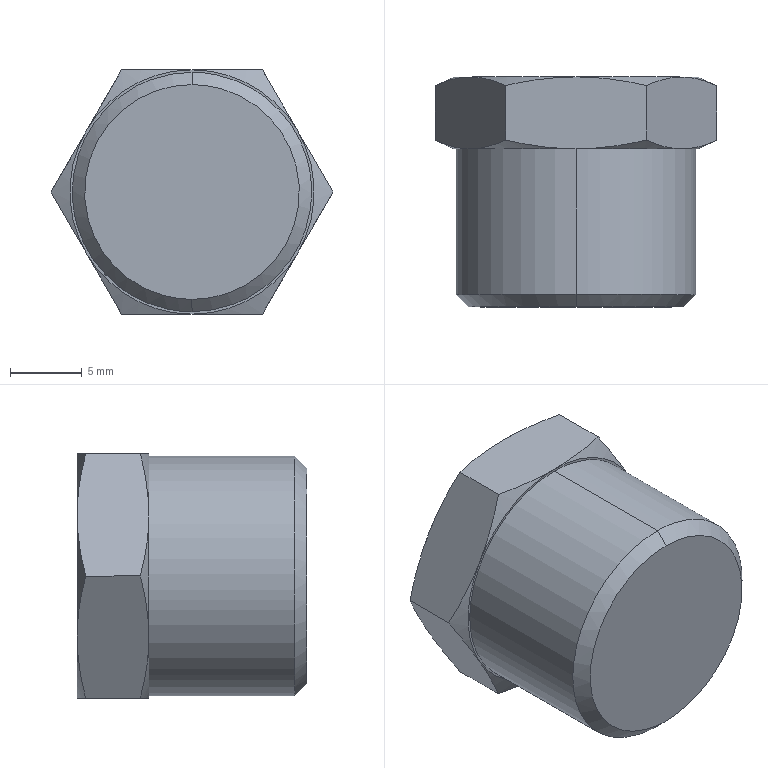Part | SolidWorks | features BaseBody 1 | 1 solid | 25 faces | box 19.63 x 16 x 17 mm | volume 3623 mm3 | cone 14 | plane 9 | cylinder 2 | commonest cylinder face diameters 16.662 x2
STEP:
#1=CARTESIAN_POINT('',(0.,0.,-7.475));
#2=VERTEX_POINT('',#1);
#3=CARTESIAN_POINT('',(0.,0.,7.475));
#4=VERTEX_POINT('',#3);
#5=CARTESIAN_POINT('',(0.,0.,-7.475));
#6=CARTESIAN_POINT('',(0.4908,0.,-7.475));
#7=CARTESIAN_POINT('',(0.9769,0.,-7.427));
#8=CARTESIAN_POINT('',(1.94,0.,-7.236));
#9=CARTESIAN_POINT('',(2.407,0.,-7.094));
#10=CARTESIAN_POINT('',(3.314,0.,-6.718));
#11=CARTESIAN_POINT('',(3.745,0.,-6.488));
#12=CARTESIAN_POINT('',(4.561,0.,-5.943));
#13=CARTESIAN_POINT('',(4.939,0.,-5.633));
#14=CARTESIAN_POINT('',(5.633,0.,-4.939));
#15=CARTESIAN_POINT('',(5.943,0.,-4.561));
#16=CARTESIAN_POINT('',(6.488,0.,-3.745));
#17=CARTESIAN_POINT('',(6.718,0.,-3.314));
#18=CARTESIAN_POINT('',(7.094,0.,-2.407));
#19=CARTESIAN_POINT('',(7.236,0.,-1.94));
#20=CARTESIAN_POINT('',(7.427,0.,-0.9769));
#21=CARTESIAN_POINT('',(7.475,0.,-0.4908));
#22=CARTESIAN_POINT('',(7.475,0.,0.4908));
#23=CARTESIAN_POINT('',(7.427,0.,0.9769));
#24=CARTESIAN_POINT('',(7.236,0.,1.94));
#25=CARTESIAN_POINT('',(7.094,0.,2.407));
#26=CARTESIAN_POINT('',(6.718,0.,3.314));
#27=CARTESIAN_POINT('',(6.488,0.,3.745));
#28=CARTESIAN_POINT('',(5.943,0.,4.561));
#29=CARTESIAN_POINT('',(5.633,0.,4.939));
#30=CARTESIAN_POINT('',(4.939,0.,5.633));
#31=CARTESIAN_POINT('',(4.561,0.,5.943));
#32=CARTESIAN_POINT('',(3.745,0.,6.488));
#33=CARTESIAN_POINT('',(3.314,0.,6.718));
#34=CARTESIAN_POINT('',(2.407,0.,7.094));
#35=CARTESIAN_POINT('',(1.94,0.,7.236));
#36=CARTESIAN_POINT('',(0.9769,0.,7.427));
#37=CARTESIAN_POINT('',(0.4908,0.,7.475));
#38=CARTESIAN_POINT('',(0.,0.,7.475));
#39=B_SPLINE_CURVE_WITH_KNOTS('',3,(#5,#6,#7,#8,#9,#10,#11,#12,#13,#14,#15,#16,#17,#18,#19,#20,#21,#22,#23,#24,#25,#26,#27,#28,#29,#30,#31,#32,#33,#34,#35,#36,#37,#38),.UNSPECIFIED.,.F.,.F.,(4,2,2,2,2,2,2,2,2,2,2,2,2,2,2,2,4),(0.,0.1963,0.3927,0.589,0.7854,0.9817,1.178,1.374,1.571,1.767,1.963,2.16,2.356,2.553,2.749,2.945,3.142),.UNSPECIFIED.);
#40=EDGE_CURVE('',#2,#4,#39,.T.);
#41=ORIENTED_EDGE('',*,*,#40,.F.);
#42=CARTESIAN_POINT('',(0.,0.856,-8.331));
#43=VERTEX_POINT('',#42);
#44=CARTESIAN_POINT('',(0.,0.856,-8.331));
#45=DIRECTION('',(0.,0.7071,-0.7071));
#46=VECTOR('',#45,1000.);
#47=LINE('',#44,#46);
#48=EDGE_CURVE('',#2,#43,#47,.T.);
#49=ORIENTED_EDGE('',*,*,#48,.T.);
#50=CARTESIAN_POINT('',(0.,0.856,8.331));
#51=VERTEX_POINT('',#50);
#52=CARTESIAN_POINT('',(0.,0.856,-8.331));
#53=CARTESIAN_POINT('',(1.091,0.856,-8.331));
#54=CARTESIAN_POINT('',(2.181,0.856,-8.114));
#55=CARTESIAN_POINT('',(4.196,0.856,-7.28));
#56=CARTESIAN_POINT('',(5.12,0.856,-6.662));
#57=CARTESIAN_POINT('',(6.662,0.856,-5.12));
#58=CARTESIAN_POINT('',(7.28,0.856,-4.196));
#59=CARTESIAN_POINT('',(8.114,0.856,-2.181));
#60=CARTESIAN_POINT('',(8.331,0.856,-1.091));
#61=CARTESIAN_POINT('',(8.331,0.856,1.091));
#62=CARTESIAN_POINT('',(8.114,0.856,2.181));
#63=CARTESIAN_POINT('',(7.28,0.856,4.196));
#64=CARTESIAN_POINT('',(6.662,0.856,5.12));
#65=CARTESIAN_POINT('',(5.12,0.856,6.662));
#66=CARTESIAN_POINT('',(4.196,0.856,7.28));
#67=CARTESIAN_POINT('',(2.181,0.856,8.114));
#68=CARTESIAN_POINT('',(1.091,0.856,8.331));
#69=CARTESIAN_POINT('',(0.,0.856,8.331));
#70=B_SPLINE_CURVE_WITH_KNOTS('',3,(#52,#53,#54,#55,#56,#57,#58,#59,#60,#61,#62,#63,#64,#65,#66,#67,#68,#69),.UNSPECIFIED.,.F.,.F.,(4,2,2,2,2,2,2,2,4),(0.,0.3927,0.7854,1.178,1.571,1.963,2.356,2.749,3.142),.UNSPECIFIED.);
#71=EDGE_CURVE('',#43,#51,#70,.T.);
#72=ORIENTED_EDGE('',*,*,#71,.T.);
#73=CARTESIAN_POINT('',(0.,0.856,8.331));
#74=DIRECTION('',(0.,0.7071,0.7071));
#75=VECTOR('',#74,1000.);
#76=LINE('',#73,#75);
#77=EDGE_CURVE('',#4,#51,#76,.T.);
#78=ORIENTED_EDGE('',*,*,#77,.F.);
#79=EDGE_LOOP('',(#41,#49,#72,#78));
#80=FACE_OUTER_BOUND('',#79,.T.);
#81=CARTESIAN_POINT('',(0.,0.856,0.));
#82=DIRECTION('',(0.,1.,0.));
#83=DIRECTION('',(0.,0.,1.));
#84=AXIS2_PLACEMENT_3D('',#81,#82,#83);
#85=CONICAL_SURFACE('',#84,8.331,0.7854);
#86=ADVANCED_FACE('',(#80),#85,.T.);
#87=CARTESIAN_POINT('',(0.,11.,-8.331));
#88=VERTEX_POINT('',#87);
#89=CARTESIAN_POINT('',(0.,11.,8.331));
#90=VERTEX_POINT('',#89);
#91=CARTESIAN_POINT('',(0.,11.,-8.331));
#92=CARTESIAN_POINT('',(1.091,11.,-8.331));
#93=CARTESIAN_POINT('',(2.181,11.,-8.114));
#94=CARTESIAN_POINT('',(4.196,11.,-7.28));
#95=CARTESIAN_POINT('',(5.12,11.,-6.662));
#96=CARTESIAN_POINT('',(6.662,11.,-5.12));
#97=CARTESIAN_POINT('',(7.28,11.,-4.196));
#98=CARTESIAN_POINT('',(8.114,11.,-2.181));
#99=CARTESIAN_POINT('',(8.331,11.,-1.091));
#100=CARTESIAN_POINT('',(8.331,11.,1.091));
#101=CARTESIAN_POINT('',(8.114,11.,2.181));
#102=CARTESIAN_POINT('',(7.28,11.,4.196));
#103=CARTESIAN_POINT('',(6.662,11.,5.12));
#104=CARTESIAN_POINT('',(5.12,11.,6.662));
#105=CARTESIAN_POINT('',(4.196,11.,7.28));
#106=CARTESIAN_POINT('',(2.181,11.,8.114));
#107=CARTESIAN_POINT('',(1.091,11.,8.331));
#108=CARTESIAN_POINT('',(0.,11.,8.331));
#109=B_SPLINE_CURVE_WITH_KNOTS('',3,(#91,#92,#93,#94,#95,#96,#97,#98,#99,#100,#101,#102,#103,#104,#105,#106,#107,#108),.UNSPECIFIED.,.F.,.F.,(4,2,2,2,2,2,2,2,4),(0.,0.3927,0.7854,1.178,1.571,1.963,2.356,2.749,3.142),.UNSPECIFIED.);
#110=EDGE_CURVE('',#88,#90,#109,.T.);
#111=ORIENTED_EDGE('',*,*,#110,.T.);
#112=CARTESIAN_POINT('',(0.,0.,8.331));
#113=DIRECTION('',(0.,-1.,0.));
#114=VECTOR('',#113,1000.);
#115=LINE('',#112,#114);
#116=EDGE_CURVE('',#90,#51,#115,.T.);
#117=ORIENTED_EDGE('',*,*,#116,.T.);
#118=ORIENTED_EDGE('',*,*,#71,.F.);
#119=CARTESIAN_POINT('',(0.,0.,-8.331));
#120=DIRECTION('',(0.,-1.,0.));
#121=VECTOR('',#120,1000.);
#122=LINE('',#119,#121);
#123=EDGE_CURVE('',#88,#43,#122,.T.);
#124=ORIENTED_EDGE('',*,*,#123,.F.);
#125=EDGE_LOOP('',(#111,#117,#118,#124));
#126=FACE_OUTER_BOUND('',#125,.T.);
#127=CARTESIAN_POINT('',(0.,0.,0.));
#128=DIRECTION('',(0.,-1.,0.));
#129=DIRECTION('',(0.,0.,-1.));
#130=AXIS2_PLACEMENT_3D('',#127,#128,#129);
#131=CYLINDRICAL_SURFACE('',#130,8.331);
#132=ADVANCED_FACE('',(#126),#131,.T.);
#133=CARTESIAN_POINT('',(-7.361,11.,4.25));
#134=VERTEX_POINT('',#133);
#135=CARTESIAN_POINT('',(-9.815,11.599,0.));
#136=VERTEX_POINT('',#135);
#137=CARTESIAN_POINT('',(-7.361,11.,4.25));
#138=CARTESIAN_POINT('',(-7.562,11.,3.903));
#139=CARTESIAN_POINT('',(-7.761,11.012,3.556));
#140=CARTESIAN_POINT('',(-8.067,11.052,3.027));
#141=CARTESIAN_POINT('',(-8.169,11.068,2.849));
#142=CARTESIAN_POINT('',(-8.326,11.098,2.578));
#143=CARTESIAN_POINT('',(-8.405,11.115,2.442));
#144=CARTESIAN_POINT('',(-8.498,11.136,2.281));
#145=CARTESIAN_POINT('',(-8.538,11.146,2.212));
#146=CARTESIAN_POINT('',(-8.565,11.152,2.165));
#147=CARTESIAN_POINT('',(-8.579,11.156,2.141));
#148=CARTESIAN_POINT('',(-8.968,11.254,1.466));
#149=CARTESIAN_POINT('',(-9.366,11.395,0.7774));
#150=CARTESIAN_POINT('',(-9.815,11.599,0.));
#151=B_SPLINE_CURVE_WITH_KNOTS('',3,(#137,#138,#139,#140,#141,#142,#143,#144,#145,#146,#147,#148,#149,#150),.UNSPECIFIED.,.F.,.F.,(4,2,2,1,1,2,2,4),(4.934,6.158,6.77,7.075,7.228,7.305,7.381,9.828),.UNSPECIFIED.);
#152=EDGE_CURVE('',#134,#136,#151,.T.);
#153=ORIENTED_EDGE('',*,*,#152,.T.);
#154=CARTESIAN_POINT('',(-7.361,11.,-4.25));
#155=VERTEX_POINT('',#154);
#156=CARTESIAN_POINT('',(-9.815,11.599,0.));
#157=CARTESIAN_POINT('',(-9.59,11.497,-0.3897));
#158=CARTESIAN_POINT('',(-9.378,11.411,-0.7558));
#159=CARTESIAN_POINT('',(-9.074,11.302,-1.282));
#160=CARTESIAN_POINT('',(-8.976,11.269,-1.453));
#161=CARTESIAN_POINT('',(-8.83,11.225,-1.705));
#162=CARTESIAN_POINT('',(-8.758,11.203,-1.83));
#163=CARTESIAN_POINT('',(-8.675,11.181,-1.974));
#164=CARTESIAN_POINT('',(-8.634,11.17,-2.046));
#165=CARTESIAN_POINT('',(-8.616,11.165,-2.076));
#166=CARTESIAN_POINT('',(-8.604,11.162,-2.097));
#167=CARTESIAN_POINT('',(-8.599,11.161,-2.105));
#168=CARTESIAN_POINT('',(-8.161,11.05,-2.864));
#169=CARTESIAN_POINT('',(-7.762,11.,-3.556));
#170=CARTESIAN_POINT('',(-7.361,11.,-4.25));
#171=B_SPLINE_CURVE_WITH_KNOTS('',3,(#156,#157,#158,#159,#160,#161,#162,#163,#164,#165,#166,#167,#168,#169,#170),.UNSPECIFIED.,.F.,.F.,(4,2,2,1,1,1,2,2,4),(0.0002337,1.234,1.85,2.159,2.313,2.39,2.429,2.467,4.934),.UNSPECIFIED.);
#172=EDGE_CURVE('',#136,#155,#171,.T.);
#173=ORIENTED_EDGE('',*,*,#172,.T.);
#174=CARTESIAN_POINT('',(0.,11.,0.));
#175=DIRECTION('',(0.,-1.,0.));
#176=DIRECTION('',(-0.866,0.,0.5));
#177=AXIS2_PLACEMENT_3D('',#174,#175,#176);
#178=CIRCLE('',#177,8.5);
#179=EDGE_CURVE('',#134,#155,#178,.T.);
#180=ORIENTED_EDGE('',*,*,#179,.F.);
#181=EDGE_LOOP('',(#153,#173,#180));
#182=FACE_OUTER_BOUND('',#181,.T.);
#183=CARTESIAN_POINT('',(0.,11.599,0.));
#184=DIRECTION('',(0.,1.,0.));
#185=DIRECTION('',(0.,0.,1.));
#186=AXIS2_PLACEMENT_3D('',#183,#184,#185);
#187=CONICAL_SURFACE('',#186,9.815,1.143);
#188=ADVANCED_FACE('',(#182),#187,.T.);
#189=CARTESIAN_POINT('',(0.,11.,-8.5));
#190=VERTEX_POINT('',#189);
#191=CARTESIAN_POINT('',(0.,11.,0.));
#192=DIRECTION('',(0.,-1.,0.));
#193=DIRECTION('',(-0.866,0.,-0.5));
#194=AXIS2_PLACEMENT_3D('',#191,#192,#193);
#195=CIRCLE('',#194,8.5);
#196=EDGE_CURVE('',#155,#190,#195,.T.);
#197=ORIENTED_EDGE('',*,*,#196,.F.);
#198=CARTESIAN_POINT('',(-4.907,11.599,-8.5));
#199=VERTEX_POINT('',#198);
#200=CARTESIAN_POINT('',(-7.361,11.,-4.25));
#201=CARTESIAN_POINT('',(-7.161,11.,-4.597));
#202=CARTESIAN_POINT('',(-6.96,11.012,-4.943));
#203=CARTESIAN_POINT('',(-6.655,11.052,-5.473));
#204=CARTESIAN_POINT('',(-6.552,11.068,-5.651));
#205=CARTESIAN_POINT('',(-6.396,11.098,-5.921));
#206=CARTESIAN_POINT('',(-6.317,11.115,-6.058));
#207=CARTESIAN_POINT('',(-6.224,11.136,-6.219));
#208=CARTESIAN_POINT('',(-6.184,11.146,-6.288));
#209=CARTESIAN_POINT('',(-6.158,11.152,-6.335));
#210=CARTESIAN_POINT('',(-6.143,11.156,-6.359));
#211=CARTESIAN_POINT('',(-5.754,11.254,-7.033));
#212=CARTESIAN_POINT('',(-5.356,11.395,-7.723));
#213=CARTESIAN_POINT('',(-4.907,11.599,-8.5));
#214=B_SPLINE_CURVE_WITH_KNOTS('',3,(#200,#201,#202,#203,#204,#205,#206,#207,#208,#209,#210,#211,#212,#213),.UNSPECIFIED.,.F.,.F.,(4,2,2,1,1,2,2,4),(4.934,6.158,6.77,7.075,7.228,7.305,7.381,9.828),.UNSPECIFIED.);
#215=EDGE_CURVE('',#155,#199,#214,.T.);
#216=ORIENTED_EDGE('',*,*,#215,.T.);
#217=CARTESIAN_POINT('',(-4.907,11.599,-8.5));
#218=CARTESIAN_POINT('',(-4.475,11.501,-8.5));
#219=CARTESIAN_POINT('',(-4.068,11.418,-8.5));
#220=CARTESIAN_POINT('',(-3.628,11.338,-8.5));
#221=CARTESIAN_POINT('',(-3.579,11.329,-8.5));
#222=CARTESIAN_POINT('',(-3.482,11.312,-8.5));
#223=CARTESIAN_POINT('',(-3.425,11.303,-8.5));
#224=CARTESIAN_POINT('',(-3.264,11.276,-8.5));
#225=CARTESIAN_POINT('',(-3.158,11.258,-8.5));
#226=CARTESIAN_POINT('',(-2.843,11.21,-8.5));
#227=CARTESIAN_POINT('',(-2.637,11.181,-8.5));
#228=CARTESIAN_POINT('',(-2.232,11.13,-8.5));
#229=CARTESIAN_POINT('',(-2.034,11.108,-8.5));
#230=CARTESIAN_POINT('',(-1.788,11.085,-8.5));
#231=CARTESIAN_POINT('',(-1.738,11.08,-8.5));
#232=CARTESIAN_POINT('',(-1.634,11.071,-8.5));
#233=CARTESIAN_POINT('',(-1.477,11.058,-8.5));
#234=CARTESIAN_POINT('',(-1.322,11.046,-8.5));
#235=CARTESIAN_POINT('',(-0.8077,11.013,-8.5));
#236=CARTESIAN_POINT('',(-0.4041,11.,-8.5));
#237=CARTESIAN_POINT('',(0.,11.,-8.5));
#238=B_SPLINE_CURVE_WITH_KNOTS('',3,(#217,#218,#219,#220,#221,#222,#223,#224,#225,#226,#227,#228,#229,#230,#231,#232,#233,#234,#235,#236,#237),.UNSPECIFIED.,.F.,.F.,(4,2,2,2,2,2,2,2,1,2,4),(10.366,11.605,11.76,11.915,12.225,12.845,13.465,13.62,13.775,14.085,15.324),.UNSPECIFIED.);
#239=EDGE_CURVE('',#199,#190,#238,.T.);
#240=ORIENTED_EDGE('',*,*,#239,.T.);
#241=EDGE_LOOP('',(#197,#216,#240));
#242=FACE_OUTER_BOUND('',#241,.T.);
#243=CARTESIAN_POINT('',(0.,11.599,0.));
#244=DIRECTION('',(0.,1.,0.));
#245=DIRECTION('',(0.,0.,1.));
#246=AXIS2_PLACEMENT_3D('',#243,#244,#245);
#247=CONICAL_SURFACE('',#246,9.815,1.143);
#248=ADVANCED_FACE('',(#242),#247,.T.);
#249=CARTESIAN_POINT('',(7.361,11.,-4.25));
#250=VERTEX_POINT('',#249);
#251=CARTESIAN_POINT('',(0.,11.,0.));
#252=DIRECTION('',(0.,-1.,0.));
#253=DIRECTION('',(0.,0.,-1.));
#254=AXIS2_PLACEMENT_3D('',#251,#252,#253);
#255=CIRCLE('',#254,8.5);
#256=EDGE_CURVE('',#190,#250,#255,.T.);
#257=ORIENTED_EDGE('',*,*,#256,.F.);
#258=CARTESIAN_POINT('',(4.907,11.599,-8.5));
#259=VERTEX_POINT('',#258);
#260=CARTESIAN_POINT('',(0.,11.,-8.5));
#261=CARTESIAN_POINT('',(0.4009,11.,-8.5));
#262=CARTESIAN_POINT('',(0.8009,11.012,-8.499));
#263=CARTESIAN_POINT('',(1.412,11.052,-8.499));
#264=CARTESIAN_POINT('',(1.617,11.068,-8.499));
#265=CARTESIAN_POINT('',(1.93,11.098,-8.5));
#266=CARTESIAN_POINT('',(2.087,11.115,-8.5));
#267=CARTESIAN_POINT('',(2.273,11.136,-8.5));
#268=CARTESIAN_POINT('',(2.367,11.147,-8.5));
#269=CARTESIAN_POINT('',(2.407,11.152,-8.5));
#270=CARTESIAN_POINT('',(2.434,11.156,-8.5));
#271=CARTESIAN_POINT('',(2.448,11.157,-8.5));
#272=CARTESIAN_POINT('',(2.657,11.184,-8.5));
#273=CARTESIAN_POINT('',(2.857,11.212,-8.5));
#274=CARTESIAN_POINT('',(3.163,11.259,-8.5));
#275=CARTESIAN_POINT('',(3.317,11.284,-8.5));
#276=CARTESIAN_POINT('',(3.5,11.315,-8.5));
#277=CARTESIAN_POINT('',(3.579,11.329,-8.5));
#278=CARTESIAN_POINT('',(3.632,11.339,-8.5));
#279=CARTESIAN_POINT('',(3.66,11.344,-8.5));
#280=CARTESIAN_POINT('',(3.785,11.366,-8.5));
#281=CARTESIAN_POINT('',(3.936,11.395,-8.5));
#282=CARTESIAN_POINT('',(4.089,11.425,-8.5));
#283=CARTESIAN_POINT('',(4.193,11.446,-8.5));
#284=CARTESIAN_POINT('',(4.246,11.456,-8.5));
#285=CARTESIAN_POINT('',(4.397,11.487,-8.5));
#286=CARTESIAN_POINT('',(4.501,11.509,-8.5));
#287=CARTESIAN_POINT('',(4.703,11.553,-8.5));
#288=CARTESIAN_POINT('',(4.805,11.576,-8.5));
#289=CARTESIAN_POINT('',(4.907,11.599,-8.5));
#290=B_SPLINE_CURVE_WITH_KNOTS('',3,(#260,#261,#262,#263,#264,#265,#266,#267,#268,#269,#270,#271,#272,#273,#274,#275,#276,#277,#278,#279,#280,#281,#282,#283,#284,#285,#286,#287,#288,#289),.UNSPECIFIED.,.F.,.F.,(4,2,2,1,1,1,2,2,2,1,1,2,2,1,2,2,2,4),(15.324,16.571,17.194,17.506,17.662,17.74,17.779,17.818,18.441,18.753,18.909,18.987,19.065,19.376,19.532,19.688,20.,20.311),.UNSPECIFIED.);
#291=EDGE_CURVE('',#190,#259,#290,.T.);
#292=ORIENTED_EDGE('',*,*,#291,.T.);
#293=CARTESIAN_POINT('',(4.907,11.599,-8.5));
#294=CARTESIAN_POINT('',(5.132,11.497,-8.11));
#295=CARTESIAN_POINT('',(5.343,11.411,-7.744));
#296=CARTESIAN_POINT('',(5.647,11.302,-7.218));
#297=CARTESIAN_POINT('',(5.746,11.269,-7.047));
#298=CARTESIAN_POINT('',(5.892,11.225,-6.794));
#299=CARTESIAN_POINT('',(5.964,11.203,-6.67));
#300=CARTESIAN_POINT('',(6.047,11.181,-6.526));
#301=CARTESIAN_POINT('',(6.089,11.17,-6.454));
#302=CARTESIAN_POINT('',(6.106,11.165,-6.424));
#303=CARTESIAN_POINT('',(6.118,11.162,-6.403));
#304=CARTESIAN_POINT('',(6.123,11.161,-6.395));
#305=CARTESIAN_POINT('',(6.561,11.05,-5.636));
#306=CARTESIAN_POINT('',(6.96,11.,-4.944));
#307=CARTESIAN_POINT('',(7.361,11.,-4.25));
#308=B_SPLINE_CURVE_WITH_KNOTS('',3,(#293,#294,#295,#296,#297,#298,#299,#300,#301,#302,#303,#304,#305,#306,#307),.UNSPECIFIED.,.F.,.F.,(4,2,2,1,1,1,2,2,4),(0.0002337,1.234,1.85,2.159,2.313,2.39,2.429,2.467,4.934),.UNSPECIFIED.);
#309=EDGE_CURVE('',#259,#250,#308,.T.);
#310=ORIENTED_EDGE('',*,*,#309,.T.);
#311=EDGE_LOOP('',(#257,#292,#310));
#312=FACE_OUTER_BOUND('',#311,.T.);
#313=CARTESIAN_POINT('',(0.,11.599,0.));
#314=DIRECTION('',(0.,1.,0.));
#315=DIRECTION('',(0.,0.,1.));
#316=AXIS2_PLACEMENT_3D('',#313,#314,#315);
#317=CONICAL_SURFACE('',#316,9.815,1.143);
#318=ADVANCED_FACE('',(#312),#317,.T.);
#319=CARTESIAN_POINT('',(7.361,11.,4.25));
#320=VERTEX_POINT('',#319);
#321=CARTESIAN_POINT('',(0.,11.,8.5));
#322=VERTEX_POINT('',#321);
#323=CARTESIAN_POINT('',(0.,11.,0.));
#324=DIRECTION('',(0.,-1.,0.));
#325=DIRECTION('',(0.866,0.,0.5));
#326=AXIS2_PLACEMENT_3D('',#323,#324,#325);
#327=CIRCLE('',#326,8.5);
#328=EDGE_CURVE('',#320,#322,#327,.T.);
#329=ORIENTED_EDGE('',*,*,#328,.F.);
#330=CARTESIAN_POINT('',(4.907,11.599,8.5));
#331=VERTEX_POINT('',#330);
#332=CARTESIAN_POINT('',(7.361,11.,4.25));
#333=CARTESIAN_POINT('',(7.161,11.,4.597));
#334=CARTESIAN_POINT('',(6.96,11.012,4.943));
#335=CARTESIAN_POINT('',(6.655,11.052,5.473));
#336=CARTESIAN_POINT('',(6.552,11.068,5.651));
#337=CARTESIAN_POINT('',(6.396,11.098,5.921));
#338=CARTESIAN_POINT('',(6.317,11.115,6.058));
#339=CARTESIAN_POINT('',(6.224,11.136,6.219));
#340=CARTESIAN_POINT('',(6.184,11.146,6.288));
#341=CARTESIAN_POINT('',(6.158,11.152,6.335));
#342=CARTESIAN_POINT('',(6.143,11.156,6.359));
#343=CARTESIAN_POINT('',(5.754,11.254,7.033));
#344=CARTESIAN_POINT('',(5.356,11.395,7.723));
#345=CARTESIAN_POINT('',(4.907,11.599,8.5));
#346=B_SPLINE_CURVE_WITH_KNOTS('',3,(#332,#333,#334,#335,#336,#337,#338,#339,#340,#341,#342,#343,#344,#345),.UNSPECIFIED.,.F.,.F.,(4,2,2,1,1,2,2,4),(4.934,6.158,6.77,7.075,7.228,7.305,7.381,9.828),.UNSPECIFIED.);
#347=EDGE_CURVE('',#320,#331,#346,.T.);
#348=ORIENTED_EDGE('',*,*,#347,.T.);
#349=CARTESIAN_POINT('',(4.907,11.599,8.5));
#350=CARTESIAN_POINT('',(4.475,11.501,8.5));
#351=CARTESIAN_POINT('',(4.068,11.418,8.5));
#352=CARTESIAN_POINT('',(3.628,11.338,8.5));
#353=CARTESIAN_POINT('',(3.579,11.329,8.5));
#354=CARTESIAN_POINT('',(3.482,11.312,8.5));
#355=CARTESIAN_POINT('',(3.425,11.303,8.5));
#356=CARTESIAN_POINT('',(3.264,11.276,8.5));
#357=CARTESIAN_POINT('',(3.158,11.258,8.5));
#358=CARTESIAN_POINT('',(2.843,11.21,8.5));
#359=CARTESIAN_POINT('',(2.637,11.181,8.5));
#360=CARTESIAN_POINT('',(2.232,11.13,8.5));
#361=CARTESIAN_POINT('',(2.034,11.108,8.5));
#362=CARTESIAN_POINT('',(1.788,11.085,8.5));
#363=CARTESIAN_POINT('',(1.738,11.08,8.5));
#364=CARTESIAN_POINT('',(1.634,11.071,8.5));
#365=CARTESIAN_POINT('',(1.477,11.058,8.5));
#366=CARTESIAN_POINT('',(1.322,11.046,8.5));
#367=CARTESIAN_POINT('',(0.8077,11.013,8.5));
#368=CARTESIAN_POINT('',(0.4041,11.,8.5));
#369=CARTESIAN_POINT('',(0.,11.,8.5));
#370=B_SPLINE_CURVE_WITH_KNOTS('',3,(#349,#350,#351,#352,#353,#354,#355,#356,#357,#358,#359,#360,#361,#362,#363,#364,#365,#366,#367,#368,#369),.UNSPECIFIED.,.F.,.F.,(4,2,2,2,2,2,2,2,1,2,4),(10.366,11.605,11.76,11.915,12.225,12.845,13.465,13.62,13.775,14.085,15.324),.UNSPECIFIED.);
#371=EDGE_CURVE('',#331,#322,#370,.T.);
#372=ORIENTED_EDGE('',*,*,#371,.T.);
#373=EDGE_LOOP('',(#329,#348,#372));
#374=FACE_OUTER_BOUND('',#373,.T.);
#375=CARTESIAN_POINT('',(0.,11.599,0.));
#376=DIRECTION('',(0.,1.,0.));
#377=DIRECTION('',(0.,0.,1.));
#378=AXIS2_PLACEMENT_3D('',#375,#376,#377);
#379=CONICAL_SURFACE('',#378,9.815,1.143);
#380=ADVANCED_FACE('',(#374),#379,.T.);
#381=CARTESIAN_POINT('',(0.,11.,0.));
#382=DIRECTION('',(0.,-1.,0.));
#383=DIRECTION('',(0.,0.,1.));
#384=AXIS2_PLACEMENT_3D('',#381,#382,#383);
#385=CIRCLE('',#384,8.5);
#386=EDGE_CURVE('',#322,#134,#385,.T.);
#387=ORIENTED_EDGE('',*,*,#386,.F.);
#388=CARTESIAN_POINT('',(-4.907,11.599,8.5));
#389=VERTEX_POINT('',#388);
#390=CARTESIAN_POINT('',(0.,11.,8.5));
#391=CARTESIAN_POINT('',(-0.4009,11.,8.5));
#392=CARTESIAN_POINT('',(-0.8009,11.012,8.499));
#393=CARTESIAN_POINT('',(-1.412,11.052,8.499));
#394=CARTESIAN_POINT('',(-1.617,11.068,8.499));
#395=CARTESIAN_POINT('',(-1.93,11.098,8.5));
#396=CARTESIAN_POINT('',(-2.087,11.115,8.5));
#397=CARTESIAN_POINT('',(-2.273,11.136,8.5));
#398=CARTESIAN_POINT('',(-2.367,11.147,8.5));
#399=CARTESIAN_POINT('',(-2.407,11.152,8.5));
#400=CARTESIAN_POINT('',(-2.434,11.156,8.5));
#401=CARTESIAN_POINT('',(-2.448,11.157,8.5));
#402=CARTESIAN_POINT('',(-2.657,11.184,8.5));
#403=CARTESIAN_POINT('',(-2.857,11.212,8.5));
#404=CARTESIAN_POINT('',(-3.163,11.259,8.5));
#405=CARTESIAN_POINT('',(-3.317,11.284,8.5));
#406=CARTESIAN_POINT('',(-3.5,11.315,8.5));
#407=CARTESIAN_POINT('',(-3.579,11.329,8.5));
#408=CARTESIAN_POINT('',(-3.632,11.339,8.5));
#409=CARTESIAN_POINT('',(-3.66,11.344,8.5));
#410=CARTESIAN_POINT('',(-3.785,11.366,8.5));
#411=CARTESIAN_POINT('',(-3.936,11.395,8.5));
#412=CARTESIAN_POINT('',(-4.089,11.425,8.5));
#413=CARTESIAN_POINT('',(-4.193,11.446,8.5));
#414=CARTESIAN_POINT('',(-4.246,11.456,8.5));
#415=CARTESIAN_POINT('',(-4.397,11.487,8.5));
#416=CARTESIAN_POINT('',(-4.501,11.509,8.5));
#417=CARTESIAN_POINT('',(-4.703,11.553,8.5));
#418=CARTESIAN_POINT('',(-4.805,11.576,8.5));
#419=CARTESIAN_POINT('',(-4.907,11.599,8.5));
#420=B_SPLINE_CURVE_WITH_KNOTS('',3,(#390,#391,#392,#393,#394,#395,#396,#397,#398,#399,#400,#401,#402,#403,#404,#405,#406,#407,#408,#409,#410,#411,#412,#413,#414,#415,#416,#417,#418,#419),.UNSPECIFIED.,.F.,.F.,(4,2,2,1,1,1,2,2,2,1,1,2,2,1,2,2,2,4),(15.324,16.571,17.194,17.506,17.662,17.74,17.779,17.818,18.441,18.753,18.909,18.987,19.065,19.376,19.532,19.688,20.,20.311),.UNSPECIFIED.);
#421=EDGE_CURVE('',#322,#389,#420,.T.);
#422=ORIENTED_EDGE('',*,*,#421,.T.);
#423=CARTESIAN_POINT('',(-4.907,11.599,8.5));
#424=CARTESIAN_POINT('',(-5.132,11.497,8.11));
#425=CARTESIAN_POINT('',(-5.343,11.411,7.744));
#426=CARTESIAN_POINT('',(-5.647,11.302,7.218));
#427=CARTESIAN_POINT('',(-5.746,11.269,7.047));
#428=CARTESIAN_POINT('',(-5.892,11.225,6.794));
#429=CARTESIAN_POINT('',(-5.964,11.203,6.67));
#430=CARTESIAN_POINT('',(-6.047,11.181,6.526));
#431=CARTESIAN_POINT('',(-6.089,11.17,6.454));
#432=CARTESIAN_POINT('',(-6.106,11.165,6.424));
#433=CARTESIAN_POINT('',(-6.118,11.162,6.403));
#434=CARTESIAN_POINT('',(-6.123,11.161,6.395));
#435=CARTESIAN_POINT('',(-6.561,11.05,5.636));
#436=CARTESIAN_POINT('',(-6.96,11.,4.944));
#437=CARTESIAN_POINT('',(-7.361,11.,4.25));
#438=B_SPLINE_CURVE_WITH_KNOTS('',3,(#423,#424,#425,#426,#427,#428,#429,#430,#431,#432,#433,#434,#435,#436,#437),.UNSPECIFIED.,.F.,.F.,(4,2,2,1,1,1,2,2,4),(0.0002337,1.234,1.85,2.159,2.313,2.39,2.429,2.467,4.934),.UNSPECIFIED.);
#439=EDGE_CURVE('',#389,#134,#438,.T.);
#440=ORIENTED_EDGE('',*,*,#439,.T.);
#441=EDGE_LOOP('',(#387,#422,#440));
#442=FACE_OUTER_BOUND('',#441,.T.);
#443=CARTESIAN_POINT('',(0.,11.599,0.));
#444=DIRECTION('',(0.,1.,0.));
#445=DIRECTION('',(0.,0.,1.));
#446=AXIS2_PLACEMENT_3D('',#443,#444,#445);
#447=CONICAL_SURFACE('',#446,9.815,1.143);
#448=ADVANCED_FACE('',(#442),#447,.T.);
#449=CARTESIAN_POINT('',(0.,11.,0.));
#450=DIRECTION('',(0.,-1.,0.));
#451=DIRECTION('',(0.866,0.,-0.5));
#452=AXIS2_PLACEMENT_3D('',#449,#450,#451);
#453=CIRCLE('',#452,8.5);
#454=EDGE_CURVE('',#250,#320,#453,.T.);
#455=ORIENTED_EDGE('',*,*,#454,.F.);
#456=CARTESIAN_POINT('',(9.815,11.599,0.));
#457=VERTEX_POINT('',#456);
#458=CARTESIAN_POINT('',(7.361,11.,-4.25));
#459=CARTESIAN_POINT('',(7.562,11.,-3.903));
#460=CARTESIAN_POINT('',(7.761,11.012,-3.556));
#461=CARTESIAN_POINT('',(8.067,11.052,-3.027));
#462=CARTESIAN_POINT('',(8.169,11.068,-2.849));
#463=CARTESIAN_POINT('',(8.326,11.098,-2.578));
#464=CARTESIAN_POINT('',(8.405,11.115,-2.442));
#465=CARTESIAN_POINT('',(8.498,11.136,-2.281));
#466=CARTESIAN_POINT('',(8.538,11.146,-2.212));
#467=CARTESIAN_POINT('',(8.565,11.152,-2.165));
#468=CARTESIAN_POINT('',(8.579,11.156,-2.141));
#469=CARTESIAN_POINT('',(8.968,11.254,-1.466));
#470=CARTESIAN_POINT('',(9.366,11.395,-0.7774));
#471=CARTESIAN_POINT('',(9.815,11.599,0.));
#472=B_SPLINE_CURVE_WITH_KNOTS('',3,(#458,#459,#460,#461,#462,#463,#464,#465,#466,#467,#468,#469,#470,#471),.UNSPECIFIED.,.F.,.F.,(4,2,2,1,1,2,2,4),(4.934,6.158,6.77,7.075,7.228,7.305,7.381,9.828),.UNSPECIFIED.);
#473=EDGE_CURVE('',#250,#457,#472,.T.);
#474=ORIENTED_EDGE('',*,*,#473,.T.);
#475=CARTESIAN_POINT('',(9.815,11.599,0.));
#476=CARTESIAN_POINT('',(9.59,11.497,0.3897));
#477=CARTESIAN_POINT('',(9.378,11.411,0.7558));
#478=CARTESIAN_POINT('',(9.074,11.302,1.282));
#479=CARTESIAN_POINT('',(8.976,11.269,1.453));
#480=CARTESIAN_POINT('',(8.83,11.225,1.705));
#481=CARTESIAN_POINT('',(8.758,11.203,1.83));
#482=CARTESIAN_POINT('',(8.675,11.181,1.974));
#483=CARTESIAN_POINT('',(8.634,11.17,2.046));
#484=CARTESIAN_POINT('',(8.616,11.165,2.076));
#485=CARTESIAN_POINT('',(8.604,11.162,2.097));
#486=CARTESIAN_POINT('',(8.599,11.161,2.105));
#487=CARTESIAN_POINT('',(8.161,11.05,2.864));
#488=CARTESIAN_POINT('',(7.762,11.,3.556));
#489=CARTESIAN_POINT('',(7.361,11.,4.25));
#490=B_SPLINE_CURVE_WITH_KNOTS('',3,(#475,#476,#477,#478,#479,#480,#481,#482,#483,#484,#485,#486,#487,#488,#489),.UNSPECIFIED.,.F.,.F.,(4,2,2,1,1,1,2,2,4),(0.0002337,1.234,1.85,2.159,2.313,2.39,2.429,2.467,4.934),.UNSPECIFIED.);
#491=EDGE_CURVE('',#457,#320,#490,.T.);
#492=ORIENTED_EDGE('',*,*,#491,.T.);
#493=EDGE_LOOP('',(#455,#474,#492));
#494=FACE_OUTER_BOUND('',#493,.T.);
#495=CARTESIAN_POINT('',(0.,11.599,0.));
#496=DIRECTION('',(0.,1.,0.));
#497=DIRECTION('',(0.,0.,1.));
#498=AXIS2_PLACEMENT_3D('',#495,#496,#497);
#499=CONICAL_SURFACE('',#498,9.815,1.143);
#500=ADVANCED_FACE('',(#494),#499,.T.);
#501=ORIENTED_EDGE('',*,*,#110,.F.);
#502=CARTESIAN_POINT('',(0.,11.,8.331));
#503=CARTESIAN_POINT('',(-1.091,11.,8.331));
#504=CARTESIAN_POINT('',(-2.181,11.,8.114));
#505=CARTESIAN_POINT('',(-4.196,11.,7.28));
#506=CARTESIAN_POINT('',(-5.12,11.,6.662));
#507=CARTESIAN_POINT('',(-6.662,11.,5.12));
#508=CARTESIAN_POINT('',(-7.28,11.,4.196));
#509=CARTESIAN_POINT('',(-8.114,11.,2.181));
#510=CARTESIAN_POINT('',(-8.331,11.,1.091));
#511=CARTESIAN_POINT('',(-8.331,11.,-1.091));
#512=CARTESIAN_POINT('',(-8.114,11.,-2.181));
#513=CARTESIAN_POINT('',(-7.28,11.,-4.196));
#514=CARTESIAN_POINT('',(-6.662,11.,-5.12));
#515=CARTESIAN_POINT('',(-5.12,11.,-6.662));
#516=CARTESIAN_POINT('',(-4.196,11.,-7.28));
#517=CARTESIAN_POINT('',(-2.181,11.,-8.114));
#518=CARTESIAN_POINT('',(-1.091,11.,-8.331));
#519=CARTESIAN_POINT('',(0.,11.,-8.331));
#520=B_SPLINE_CURVE_WITH_KNOTS('',3,(#502,#503,#504,#505,#506,#507,#508,#509,#510,#511,#512,#513,#514,#515,#516,#517,#518,#519),.UNSPECIFIED.,.F.,.F.,(4,2,2,2,2,2,2,2,4),(3.142,3.534,3.927,4.32,4.712,5.105,5.498,5.89,6.283),.UNSPECIFIED.);
#521=EDGE_CURVE('',#90,#88,#520,.T.);
#522=ORIENTED_EDGE('',*,*,#521,.F.);
#523=EDGE_LOOP('',(#501,#522));
#524=FACE_BOUND('',#523,.T.);
#525=ORIENTED_EDGE('',*,*,#256,.T.);
#526=ORIENTED_EDGE('',*,*,#454,.T.);
#527=ORIENTED_EDGE('',*,*,#328,.T.);
#528=ORIENTED_EDGE('',*,*,#386,.T.);
#529=ORIENTED_EDGE('',*,*,#179,.T.);
#530=ORIENTED_EDGE('',*,*,#196,.T.);
#531=EDGE_LOOP('',(#525,#526,#527,#528,#529,#530));
#532=FACE_OUTER_BOUND('',#531,.T.);
#533=CARTESIAN_POINT('',(8.5,11.,0.));
#534=DIRECTION('',(0.,1.,0.));
#535=DIRECTION('',(0.,0.,1.));
#536=AXIS2_PLACEMENT_3D('',#533,#534,#535);
#537=PLANE('',#536);
#538=ADVANCED_FACE('',(#524,#532),#537,.F.);
#539=ORIENTED_EDGE('',*,*,#116,.F.);
#540=ORIENTED_EDGE('',*,*,#521,.T.);
#541=ORIENTED_EDGE('',*,*,#123,.T.);
#542=CARTESIAN_POINT('',(0.,0.856,8.331));
#543=CARTESIAN_POINT('',(-1.091,0.856,8.331));
#544=CARTESIAN_POINT('',(-2.181,0.856,8.114));
#545=CARTESIAN_POINT('',(-4.196,0.856,7.28));
#546=CARTESIAN_POINT('',(-5.12,0.856,6.662));
#547=CARTESIAN_POINT('',(-6.662,0.856,5.12));
#548=CARTESIAN_POINT('',(-7.28,0.856,4.196));
#549=CARTESIAN_POINT('',(-8.114,0.856,2.181));
#550=CARTESIAN_POINT('',(-8.331,0.856,1.091));
#551=CARTESIAN_POINT('',(-8.331,0.856,-1.091));
#552=CARTESIAN_POINT('',(-8.114,0.856,-2.181));
#553=CARTESIAN_POINT('',(-7.28,0.856,-4.196));
#554=CARTESIAN_POINT('',(-6.662,0.856,-5.12));
#555=CARTESIAN_POINT('',(-5.12,0.856,-6.662));
#556=CARTESIAN_POINT('',(-4.196,0.856,-7.28));
#557=CARTESIAN_POINT('',(-2.181,0.856,-8.114));
#558=CARTESIAN_POINT('',(-1.091,0.856,-8.331));
#559=CARTESIAN_POINT('',(0.,0.856,-8.331));
#560=B_SPLINE_CURVE_WITH_KNOTS('',3,(#542,#543,#544,#545,#546,#547,#548,#549,#550,#551,#552,#553,#554,#555,#556,#557,#558,#559),.UNSPECIFIED.,.F.,.F.,(4,2,2,2,2,2,2,2,4),(3.142,3.534,3.927,4.32,4.712,5.105,5.498,5.89,6.283),.UNSPECIFIED.);
#561=EDGE_CURVE('',#51,#43,#560,.T.);
#562=ORIENTED_EDGE('',*,*,#561,.F.);
#563=EDGE_LOOP('',(#539,#540,#541,#562));
#564=FACE_OUTER_BOUND('',#563,.T.);
#565=CARTESIAN_POINT('',(0.,0.,0.));
#566=DIRECTION('',(0.,-1.,0.));
#567=DIRECTION('',(0.,0.,-1.));
#568=AXIS2_PLACEMENT_3D('',#565,#566,#567);
#569=CYLINDRICAL_SURFACE('',#568,8.331);
#570=ADVANCED_FACE('',(#564),#569,.T.);
#571=ORIENTED_EDGE('',*,*,#48,.F.);
#572=CARTESIAN_POINT('',(0.,0.,7.475));
#573=CARTESIAN_POINT('',(-0.4908,0.,7.475));
#574=CARTESIAN_POINT('',(-0.9769,0.,7.427));
#575=CARTESIAN_POINT('',(-1.94,0.,7.236));
#576=CARTESIAN_POINT('',(-2.407,0.,7.094));
#577=CARTESIAN_POINT('',(-3.314,0.,6.718));
#578=CARTESIAN_POINT('',(-3.745,0.,6.488));
#579=CARTESIAN_POINT('',(-4.561,0.,5.943));
#580=CARTESIAN_POINT('',(-4.939,0.,5.633));
#581=CARTESIAN_POINT('',(-5.633,0.,4.939));
#582=CARTESIAN_POINT('',(-5.943,0.,4.561));
#583=CARTESIAN_POINT('',(-6.488,0.,3.745));
#584=CARTESIAN_POINT('',(-6.718,0.,3.314));
#585=CARTESIAN_POINT('',(-7.094,0.,2.407));
#586=CARTESIAN_POINT('',(-7.236,0.,1.94));
#587=CARTESIAN_POINT('',(-7.427,0.,0.9769));
#588=CARTESIAN_POINT('',(-7.475,0.,0.4908));
#589=CARTESIAN_POINT('',(-7.475,0.,-0.4908));
#590=CARTESIAN_POINT('',(-7.427,0.,-0.9769));
#591=CARTESIAN_POINT('',(-7.236,0.,-1.94));
#592=CARTESIAN_POINT('',(-7.094,0.,-2.407));
#593=CARTESIAN_POINT('',(-6.718,0.,-3.314));
#594=CARTESIAN_POINT('',(-6.488,0.,-3.745));
#595=CARTESIAN_POINT('',(-5.943,0.,-4.561));
#596=CARTESIAN_POINT('',(-5.633,0.,-4.939));
#597=CARTESIAN_POINT('',(-4.939,0.,-5.633));
#598=CARTESIAN_POINT('',(-4.561,0.,-5.943));
#599=CARTESIAN_POINT('',(-3.745,0.,-6.488));
#600=CARTESIAN_POINT('',(-3.314,0.,-6.718));
#601=CARTESIAN_POINT('',(-2.407,0.,-7.094));
#602=CARTESIAN_POINT('',(-1.94,0.,-7.236));
#603=CARTESIAN_POINT('',(-0.9769,0.,-7.427));
#604=CARTESIAN_POINT('',(-0.4908,0.,-7.475));
#605=CARTESIAN_POINT('',(0.,0.,-7.475));
#606=B_SPLINE_CURVE_WITH_KNOTS('',3,(#572,#573,#574,#575,#576,#577,#578,#579,#580,#581,#582,#583,#584,#585,#586,#587,#588,#589,#590,#591,#592,#593,#594,#595,#596,#597,#598,#599,#600,#601,#602,#603,#604,#605),.UNSPECIFIED.,.F.,.F.,(4,2,2,2,2,2,2,2,2,2,2,2,2,2,2,2,4),(3.142,3.338,3.534,3.731,3.927,4.123,4.32,4.516,4.712,4.909,5.105,5.301,5.498,5.694,5.89,6.087,6.283),.UNSPECIFIED.);
#607=EDGE_CURVE('',#4,#2,#606,.T.);
#608=ORIENTED_EDGE('',*,*,#607,.F.);
#609=ORIENTED_EDGE('',*,*,#77,.T.);
#610=ORIENTED_EDGE('',*,*,#561,.T.);
#611=EDGE_LOOP('',(#571,#608,#609,#610));
#612=FACE_OUTER_BOUND('',#611,.T.);
#613=CARTESIAN_POINT('',(0.,0.856,0.));
#614=DIRECTION('',(0.,1.,0.));
#615=DIRECTION('',(0.,0.,1.));
#616=AXIS2_PLACEMENT_3D('',#613,#614,#615);
#617=CONICAL_SURFACE('',#616,8.331,0.7854);
#618=ADVANCED_FACE('',(#612),#617,.T.);
#619=ORIENTED_EDGE('',*,*,#607,.T.);
#620=ORIENTED_EDGE('',*,*,#40,.T.);
#621=EDGE_LOOP('',(#619,#620));
#622=FACE_OUTER_BOUND('',#621,.T.);
#623=CARTESIAN_POINT('',(7.475,0.,0.));
#624=DIRECTION('',(0.,1.,0.));
#625=DIRECTION('',(0.,0.,1.));
#626=AXIS2_PLACEMENT_3D('',#623,#624,#625);
#627=PLANE('',#626);
#628=ADVANCED_FACE('',(#622),#627,.F.);
#629=CARTESIAN_POINT('',(-4.907,15.401,-8.5));
#630=VERTEX_POINT('',#629);
#631=CARTESIAN_POINT('',(-4.907,15.401,-8.5));
#632=DIRECTION('',(0.,-1.,0.));
#633=VECTOR('',#632,1000.);
#634=LINE('',#631,#633);
#635=EDGE_CURVE('',#630,#199,#634,.T.);
#636=ORIENTED_EDGE('',*,*,#635,.T.);
#637=ORIENTED_EDGE('',*,*,#215,.F.);
#638=ORIENTED_EDGE('',*,*,#172,.F.);
#639=CARTESIAN_POINT('',(-9.815,15.401,0.));
#640=VERTEX_POINT('',#639);
#641=CARTESIAN_POINT('',(-9.815,15.401,0.));
#642=DIRECTION('',(0.,-1.,0.));
#643=VECTOR('',#642,1000.);
#644=LINE('',#641,#643);
#645=EDGE_CURVE('',#640,#136,#644,.T.);
#646=ORIENTED_EDGE('',*,*,#645,.F.);
#647=CARTESIAN_POINT('',(-7.361,16.,-4.25));
#648=VERTEX_POINT('',#647);
#649=CARTESIAN_POINT('',(-7.361,16.,-4.25));
#650=CARTESIAN_POINT('',(-7.562,16.,-3.903));
#651=CARTESIAN_POINT('',(-7.761,15.988,-3.556));
#652=CARTESIAN_POINT('',(-8.067,15.948,-3.027));
#653=CARTESIAN_POINT('',(-8.169,15.932,-2.849));
#654=CARTESIAN_POINT('',(-8.326,15.902,-2.578));
#655=CARTESIAN_POINT('',(-8.405,15.885,-2.442));
#656=CARTESIAN_POINT('',(-8.498,15.864,-2.281));
#657=CARTESIAN_POINT('',(-8.538,15.854,-2.212));
#658=CARTESIAN_POINT('',(-8.565,15.848,-2.165));
#659=CARTESIAN_POINT('',(-8.579,15.844,-2.141));
#660=CARTESIAN_POINT('',(-8.968,15.746,-1.466));
#661=CARTESIAN_POINT('',(-9.366,15.605,-0.7774));
#662=CARTESIAN_POINT('',(-9.815,15.401,0.));
#663=B_SPLINE_CURVE_WITH_KNOTS('',3,(#649,#650,#651,#652,#653,#654,#655,#656,#657,#658,#659,#660,#661,#662),.UNSPECIFIED.,.F.,.F.,(4,2,2,1,1,2,2,4),(4.934,6.158,6.77,7.075,7.228,7.305,7.381,9.828),.UNSPECIFIED.);
#664=EDGE_CURVE('',#648,#640,#663,.T.);
#665=ORIENTED_EDGE('',*,*,#664,.F.);
#666=CARTESIAN_POINT('',(-4.907,15.401,-8.5));
#667=CARTESIAN_POINT('',(-5.132,15.503,-8.11));
#668=CARTESIAN_POINT('',(-5.343,15.589,-7.744));
#669=CARTESIAN_POINT('',(-5.647,15.698,-7.218));
#670=CARTESIAN_POINT('',(-5.746,15.731,-7.047));
#671=CARTESIAN_POINT('',(-5.892,15.775,-6.794));
#672=CARTESIAN_POINT('',(-5.964,15.797,-6.67));
#673=CARTESIAN_POINT('',(-6.047,15.819,-6.526));
#674=CARTESIAN_POINT('',(-6.089,15.83,-6.454));
#675=CARTESIAN_POINT('',(-6.106,15.835,-6.424));
#676=CARTESIAN_POINT('',(-6.118,15.838,-6.403));
#677=CARTESIAN_POINT('',(-6.123,15.839,-6.395));
#678=CARTESIAN_POINT('',(-6.561,15.95,-5.636));
#679=CARTESIAN_POINT('',(-6.96,16.,-4.944));
#680=CARTESIAN_POINT('',(-7.361,16.,-4.25));
#681=B_SPLINE_CURVE_WITH_KNOTS('',3,(#666,#667,#668,#669,#670,#671,#672,#673,#674,#675,#676,#677,#678,#679,#680),.UNSPECIFIED.,.F.,.F.,(4,2,2,1,1,1,2,2,4),(0.0002337,1.234,1.85,2.159,2.313,2.39,2.429,2.467,4.934),.UNSPECIFIED.);
#682=EDGE_CURVE('',#630,#648,#681,.T.);
#683=ORIENTED_EDGE('',*,*,#682,.F.);
#684=EDGE_LOOP('',(#636,#637,#638,#646,#665,#683));
#685=FACE_OUTER_BOUND('',#684,.T.);
#686=CARTESIAN_POINT('',(-4.907,16.,-8.5));
#687=DIRECTION('',(0.866,0.,0.5));
#688=DIRECTION('',(0.5,0.,-0.866));
#689=AXIS2_PLACEMENT_3D('',#686,#687,#688);
#690=PLANE('',#689);
#691=ADVANCED_FACE('',(#685),#690,.F.);
#692=CARTESIAN_POINT('',(4.907,15.401,-8.5));
#693=VERTEX_POINT('',#692);
#694=CARTESIAN_POINT('',(4.907,15.401,-8.5));
#695=DIRECTION('',(0.,-1.,0.));
#696=VECTOR('',#695,1000.);
#697=LINE('',#694,#696);
#698=EDGE_CURVE('',#693,#259,#697,.T.);
#699=ORIENTED_EDGE('',*,*,#698,.T.);
#700=ORIENTED_EDGE('',*,*,#291,.F.);
#701=ORIENTED_EDGE('',*,*,#239,.F.);
#702=ORIENTED_EDGE('',*,*,#635,.F.);
#703=CARTESIAN_POINT('',(0.,16.,-8.5));
#704=VERTEX_POINT('',#703);
#705=CARTESIAN_POINT('',(0.,16.,-8.5));
#706=CARTESIAN_POINT('',(-0.4009,16.,-8.5));
#707=CARTESIAN_POINT('',(-0.8009,15.988,-8.499));
#708=CARTESIAN_POINT('',(-1.412,15.948,-8.499));
#709=CARTESIAN_POINT('',(-1.617,15.932,-8.499));
#710=CARTESIAN_POINT('',(-1.93,15.902,-8.5));
#711=CARTESIAN_POINT('',(-2.087,15.885,-8.5));
#712=CARTESIAN_POINT('',(-2.273,15.864,-8.5));
#713=CARTESIAN_POINT('',(-2.367,15.853,-8.5));
#714=CARTESIAN_POINT('',(-2.407,15.848,-8.5));
#715=CARTESIAN_POINT('',(-2.434,15.844,-8.5));
#716=CARTESIAN_POINT('',(-2.448,15.843,-8.5));
#717=CARTESIAN_POINT('',(-2.657,15.816,-8.5));
#718=CARTESIAN_POINT('',(-2.857,15.788,-8.5));
#719=CARTESIAN_POINT('',(-3.163,15.741,-8.5));
#720=CARTESIAN_POINT('',(-3.317,15.716,-8.5));
#721=CARTESIAN_POINT('',(-3.5,15.685,-8.5));
#722=CARTESIAN_POINT('',(-3.579,15.671,-8.5));
#723=CARTESIAN_POINT('',(-3.632,15.661,-8.5));
#724=CARTESIAN_POINT('',(-3.66,15.656,-8.5));
#725=CARTESIAN_POINT('',(-3.785,15.634,-8.5));
#726=CARTESIAN_POINT('',(-3.936,15.605,-8.5));
#727=CARTESIAN_POINT('',(-4.089,15.575,-8.5));
#728=CARTESIAN_POINT('',(-4.193,15.554,-8.5));
#729=CARTESIAN_POINT('',(-4.246,15.544,-8.5));
#730=CARTESIAN_POINT('',(-4.397,15.513,-8.5));
#731=CARTESIAN_POINT('',(-4.501,15.491,-8.5));
#732=CARTESIAN_POINT('',(-4.703,15.447,-8.5));
#733=CARTESIAN_POINT('',(-4.805,15.424,-8.5));
#734=CARTESIAN_POINT('',(-4.907,15.401,-8.5));
#735=B_SPLINE_CURVE_WITH_KNOTS('',3,(#705,#706,#707,#708,#709,#710,#711,#712,#713,#714,#715,#716,#717,#718,#719,#720,#721,#722,#723,#724,#725,#726,#727,#728,#729,#730,#731,#732,#733,#734),.UNSPECIFIED.,.F.,.F.,(4,2,2,1,1,1,2,2,2,1,1,2,2,1,2,2,2,4),(15.324,16.571,17.194,17.506,17.662,17.74,17.779,17.818,18.441,18.753,18.909,18.987,19.065,19.376,19.532,19.688,20.,20.311),.UNSPECIFIED.);
#736=EDGE_CURVE('',#704,#630,#735,.T.);
#737=ORIENTED_EDGE('',*,*,#736,.F.);
#738=CARTESIAN_POINT('',(4.907,15.401,-8.5));
#739=CARTESIAN_POINT('',(4.475,15.499,-8.5));
#740=CARTESIAN_POINT('',(4.068,15.582,-8.5));
#741=CARTESIAN_POINT('',(3.628,15.662,-8.5));
#742=CARTESIAN_POINT('',(3.579,15.671,-8.5));
#743=CARTESIAN_POINT('',(3.482,15.688,-8.5));
#744=CARTESIAN_POINT('',(3.425,15.697,-8.5));
#745=CARTESIAN_POINT('',(3.264,15.724,-8.5));
#746=CARTESIAN_POINT('',(3.158,15.742,-8.5));
#747=CARTESIAN_POINT('',(2.843,15.79,-8.5));
#748=CARTESIAN_POINT('',(2.637,15.819,-8.5));
#749=CARTESIAN_POINT('',(2.232,15.87,-8.5));
#750=CARTESIAN_POINT('',(2.034,15.892,-8.5));
#751=CARTESIAN_POINT('',(1.788,15.915,-8.5));
#752=CARTESIAN_POINT('',(1.738,15.92,-8.5));
#753=CARTESIAN_POINT('',(1.634,15.929,-8.5));
#754=CARTESIAN_POINT('',(1.477,15.942,-8.5));
#755=CARTESIAN_POINT('',(1.322,15.954,-8.5));
#756=CARTESIAN_POINT('',(0.8077,15.987,-8.5));
#757=CARTESIAN_POINT('',(0.4041,16.,-8.5));
#758=CARTESIAN_POINT('',(0.,16.,-8.5));
#759=B_SPLINE_CURVE_WITH_KNOTS('',3,(#738,#739,#740,#741,#742,#743,#744,#745,#746,#747,#748,#749,#750,#751,#752,#753,#754,#755,#756,#757,#758),.UNSPECIFIED.,.F.,.F.,(4,2,2,2,2,2,2,2,1,2,4),(10.366,11.605,11.76,11.915,12.225,12.845,13.465,13.62,13.775,14.085,15.324),.UNSPECIFIED.);
#760=EDGE_CURVE('',#693,#704,#759,.T.);
#761=ORIENTED_EDGE('',*,*,#760,.F.);
#762=EDGE_LOOP('',(#699,#700,#701,#702,#737,#761));
#763=FACE_OUTER_BOUND('',#762,.T.);
#764=CARTESIAN_POINT('',(4.907,16.,-8.5));
#765=DIRECTION('',(0.,0.,1.));
#766=DIRECTION('',(1.,0.,0.));
#767=AXIS2_PLACEMENT_3D('',#764,#765,#766);
#768=PLANE('',#767);
#769=ADVANCED_FACE('',(#763),#768,.F.);
#770=CARTESIAN_POINT('',(9.815,15.401,0.));
#771=VERTEX_POINT('',#770);
#772=CARTESIAN_POINT('',(9.815,15.401,0.));
#773=DIRECTION('',(0.,-1.,0.));
#774=VECTOR('',#773,1000.);
#775=LINE('',#772,#774);
#776=EDGE_CURVE('',#771,#457,#775,.T.);
#777=ORIENTED_EDGE('',*,*,#776,.T.);
#778=ORIENTED_EDGE('',*,*,#473,.F.);
#779=ORIENTED_EDGE('',*,*,#309,.F.);
#780=ORIENTED_EDGE('',*,*,#698,.F.);
#781=CARTESIAN_POINT('',(7.361,16.,-4.25));
#782=VERTEX_POINT('',#781);
#783=CARTESIAN_POINT('',(7.361,16.,-4.25));
#784=CARTESIAN_POINT('',(7.161,16.,-4.597));
#785=CARTESIAN_POINT('',(6.96,15.988,-4.943));
#786=CARTESIAN_POINT('',(6.655,15.948,-5.473));
#787=CARTESIAN_POINT('',(6.552,15.932,-5.651));
#788=CARTESIAN_POINT('',(6.396,15.902,-5.921));
#789=CARTESIAN_POINT('',(6.317,15.885,-6.058));
#790=CARTESIAN_POINT('',(6.224,15.864,-6.219));
#791=CARTESIAN_POINT('',(6.184,15.854,-6.288));
#792=CARTESIAN_POINT('',(6.158,15.848,-6.335));
#793=CARTESIAN_POINT('',(6.143,15.844,-6.359));
#794=CARTESIAN_POINT('',(5.754,15.746,-7.033));
#795=CARTESIAN_POINT('',(5.356,15.605,-7.723));
#796=CARTESIAN_POINT('',(4.907,15.401,-8.5));
#797=B_SPLINE_CURVE_WITH_KNOTS('',3,(#783,#784,#785,#786,#787,#788,#789,#790,#791,#792,#793,#794,#795,#796),.UNSPECIFIED.,.F.,.F.,(4,2,2,1,1,2,2,4),(4.934,6.158,6.77,7.075,7.228,7.305,7.381,9.828),.UNSPECIFIED.);
#798=EDGE_CURVE('',#782,#693,#797,.T.);
#799=ORIENTED_EDGE('',*,*,#798,.F.);
#800=CARTESIAN_POINT('',(9.815,15.401,0.));
#801=CARTESIAN_POINT('',(9.59,15.503,-0.3897));
#802=CARTESIAN_POINT('',(9.378,15.589,-0.7558));
#803=CARTESIAN_POINT('',(9.074,15.698,-1.282));
#804=CARTESIAN_POINT('',(8.976,15.731,-1.453));
#805=CARTESIAN_POINT('',(8.83,15.775,-1.705));
#806=CARTESIAN_POINT('',(8.758,15.797,-1.83));
#807=CARTESIAN_POINT('',(8.675,15.819,-1.974));
#808=CARTESIAN_POINT('',(8.634,15.83,-2.046));
#809=CARTESIAN_POINT('',(8.616,15.835,-2.076));
#810=CARTESIAN_POINT('',(8.604,15.838,-2.097));
#811=CARTESIAN_POINT('',(8.599,15.839,-2.105));
#812=CARTESIAN_POINT('',(8.161,15.95,-2.864));
#813=CARTESIAN_POINT('',(7.762,16.,-3.556));
#814=CARTESIAN_POINT('',(7.361,16.,-4.25));
#815=B_SPLINE_CURVE_WITH_KNOTS('',3,(#800,#801,#802,#803,#804,#805,#806,#807,#808,#809,#810,#811,#812,#813,#814),.UNSPECIFIED.,.F.,.F.,(4,2,2,1,1,1,2,2,4),(0.0002337,1.234,1.85,2.159,2.313,2.39,2.429,2.467,4.934),.UNSPECIFIED.);
#816=EDGE_CURVE('',#771,#782,#815,.T.);
#817=ORIENTED_EDGE('',*,*,#816,.F.);
#818=EDGE_LOOP('',(#777,#778,#779,#780,#799,#817));
#819=FACE_OUTER_BOUND('',#818,.T.);
#820=CARTESIAN_POINT('',(9.815,16.,0.));
#821=DIRECTION('',(-0.866,0.,0.5));
#822=DIRECTION('',(0.5,0.,0.866));
#823=AXIS2_PLACEMENT_3D('',#820,#821,#822);
#824=PLANE('',#823);
#825=ADVANCED_FACE('',(#819),#824,.F.);
#826=CARTESIAN_POINT('',(4.907,15.401,8.5));
#827=VERTEX_POINT('',#826);
#828=CARTESIAN_POINT('',(4.907,15.401,8.5));
#829=DIRECTION('',(0.,-1.,0.));
#830=VECTOR('',#829,1000.);
#831=LINE('',#828,#830);
#832=EDGE_CURVE('',#827,#331,#831,.T.);
#833=ORIENTED_EDGE('',*,*,#832,.T.);
#834=ORIENTED_EDGE('',*,*,#347,.F.);
#835=ORIENTED_EDGE('',*,*,#491,.F.);
#836=ORIENTED_EDGE('',*,*,#776,.F.);
#837=CARTESIAN_POINT('',(7.361,16.,4.25));
#838=VERTEX_POINT('',#837);
#839=CARTESIAN_POINT('',(7.361,16.,4.25));
#840=CARTESIAN_POINT('',(7.562,16.,3.903));
#841=CARTESIAN_POINT('',(7.761,15.988,3.556));
#842=CARTESIAN_POINT('',(8.067,15.948,3.027));
#843=CARTESIAN_POINT('',(8.169,15.932,2.849));
#844=CARTESIAN_POINT('',(8.326,15.902,2.578));
#845=CARTESIAN_POINT('',(8.405,15.885,2.442));
#846=CARTESIAN_POINT('',(8.498,15.864,2.281));
#847=CARTESIAN_POINT('',(8.538,15.854,2.212));
#848=CARTESIAN_POINT('',(8.565,15.848,2.165));
#849=CARTESIAN_POINT('',(8.579,15.844,2.141));
#850=CARTESIAN_POINT('',(8.968,15.746,1.466));
#851=CARTESIAN_POINT('',(9.366,15.605,0.7774));
#852=CARTESIAN_POINT('',(9.815,15.401,0.));
#853=B_SPLINE_CURVE_WITH_KNOTS('',3,(#839,#840,#841,#842,#843,#844,#845,#846,#847,#848,#849,#850,#851,#852),.UNSPECIFIED.,.F.,.F.,(4,2,2,1,1,2,2,4),(4.934,6.158,6.77,7.075,7.228,7.305,7.381,9.828),.UNSPECIFIED.);
#854=EDGE_CURVE('',#838,#771,#853,.T.);
#855=ORIENTED_EDGE('',*,*,#854,.F.);
#856=CARTESIAN_POINT('',(4.907,15.401,8.5));
#857=CARTESIAN_POINT('',(5.132,15.503,8.11));
#858=CARTESIAN_POINT('',(5.343,15.589,7.744));
#859=CARTESIAN_POINT('',(5.647,15.698,7.218));
#860=CARTESIAN_POINT('',(5.746,15.731,7.047));
#861=CARTESIAN_POINT('',(5.892,15.775,6.794));
#862=CARTESIAN_POINT('',(5.964,15.797,6.67));
#863=CARTESIAN_POINT('',(6.047,15.819,6.526));
#864=CARTESIAN_POINT('',(6.089,15.83,6.454));
#865=CARTESIAN_POINT('',(6.106,15.835,6.424));
#866=CARTESIAN_POINT('',(6.118,15.838,6.403));
#867=CARTESIAN_POINT('',(6.123,15.839,6.395));
#868=CARTESIAN_POINT('',(6.561,15.95,5.636));
#869=CARTESIAN_POINT('',(6.96,16.,4.944));
#870=CARTESIAN_POINT('',(7.361,16.,4.25));
#871=B_SPLINE_CURVE_WITH_KNOTS('',3,(#856,#857,#858,#859,#860,#861,#862,#863,#864,#865,#866,#867,#868,#869,#870),.UNSPECIFIED.,.F.,.F.,(4,2,2,1,1,1,2,2,4),(0.0002337,1.234,1.85,2.159,2.313,2.39,2.429,2.467,4.934),.UNSPECIFIED.);
#872=EDGE_CURVE('',#827,#838,#871,.T.);
#873=ORIENTED_EDGE('',*,*,#872,.F.);
#874=EDGE_LOOP('',(#833,#834,#835,#836,#855,#873));
#875=FACE_OUTER_BOUND('',#874,.T.);
#876=CARTESIAN_POINT('',(4.907,16.,8.5));
#877=DIRECTION('',(-0.866,0.,-0.5));
#878=DIRECTION('',(-0.5,0.,0.866));
#879=AXIS2_PLACEMENT_3D('',#876,#877,#878);
#880=PLANE('',#879);
#881=ADVANCED_FACE('',(#875),#880,.F.);
#882=CARTESIAN_POINT('',(-4.907,15.401,8.5));
#883=VERTEX_POINT('',#882);
#884=CARTESIAN_POINT('',(-4.907,15.401,8.5));
#885=DIRECTION('',(0.,-1.,0.));
#886=VECTOR('',#885,1000.);
#887=LINE('',#884,#886);
#888=EDGE_CURVE('',#883,#389,#887,.T.);
#889=ORIENTED_EDGE('',*,*,#888,.T.);
#890=ORIENTED_EDGE('',*,*,#421,.F.);
#891=ORIENTED_EDGE('',*,*,#371,.F.);
#892=ORIENTED_EDGE('',*,*,#832,.F.);
#893=CARTESIAN_POINT('',(0.,16.,8.5));
#894=VERTEX_POINT('',#893);
#895=CARTESIAN_POINT('',(0.,16.,8.5));
#896=CARTESIAN_POINT('',(0.4009,16.,8.5));
#897=CARTESIAN_POINT('',(0.8009,15.988,8.499));
#898=CARTESIAN_POINT('',(1.412,15.948,8.499));
#899=CARTESIAN_POINT('',(1.617,15.932,8.499));
#900=CARTESIAN_POINT('',(1.93,15.902,8.5));
#901=CARTESIAN_POINT('',(2.087,15.885,8.5));
#902=CARTESIAN_POINT('',(2.273,15.864,8.5));
#903=CARTESIAN_POINT('',(2.367,15.853,8.5));
#904=CARTESIAN_POINT('',(2.407,15.848,8.5));
#905=CARTESIAN_POINT('',(2.434,15.844,8.5));
#906=CARTESIAN_POINT('',(2.448,15.843,8.5));
#907=CARTESIAN_POINT('',(2.657,15.816,8.5));
#908=CARTESIAN_POINT('',(2.857,15.788,8.5));
#909=CARTESIAN_POINT('',(3.163,15.741,8.5));
#910=CARTESIAN_POINT('',(3.317,15.716,8.5));
#911=CARTESIAN_POINT('',(3.5,15.685,8.5));
#912=CARTESIAN_POINT('',(3.579,15.671,8.5));
#913=CARTESIAN_POINT('',(3.632,15.661,8.5));
#914=CARTESIAN_POINT('',(3.66,15.656,8.5));
#915=CARTESIAN_POINT('',(3.785,15.634,8.5));
#916=CARTESIAN_POINT('',(3.936,15.605,8.5));
#917=CARTESIAN_POINT('',(4.089,15.575,8.5));
#918=CARTESIAN_POINT('',(4.193,15.554,8.5));
#919=CARTESIAN_POINT('',(4.246,15.544,8.5));
#920=CARTESIAN_POINT('',(4.397,15.513,8.5));
#921=CARTESIAN_POINT('',(4.501,15.491,8.5));
#922=CARTESIAN_POINT('',(4.703,15.447,8.5));
#923=CARTESIAN_POINT('',(4.805,15.424,8.5));
#924=CARTESIAN_POINT('',(4.907,15.401,8.5));
#925=B_SPLINE_CURVE_WITH_KNOTS('',3,(#895,#896,#897,#898,#899,#900,#901,#902,#903,#904,#905,#906,#907,#908,#909,#910,#911,#912,#913,#914,#915,#916,#917,#918,#919,#920,#921,#922,#923,#924),.UNSPECIFIED.,.F.,.F.,(4,2,2,1,1,1,2,2,2,1,1,2,2,1,2,2,2,4),(15.324,16.571,17.194,17.506,17.662,17.74,17.779,17.818,18.441,18.753,18.909,18.987,19.065,19.376,19.532,19.688,20.,20.311),.UNSPECIFIED.);
#926=EDGE_CURVE('',#894,#827,#925,.T.);
#927=ORIENTED_EDGE('',*,*,#926,.F.);
#928=CARTESIAN_POINT('',(-4.907,15.401,8.5));
#929=CARTESIAN_POINT('',(-4.475,15.499,8.5));
#930=CARTESIAN_POINT('',(-4.068,15.582,8.5));
#931=CARTESIAN_POINT('',(-3.628,15.662,8.5));
#932=CARTESIAN_POINT('',(-3.579,15.671,8.5));
#933=CARTESIAN_POINT('',(-3.482,15.688,8.5));
#934=CARTESIAN_POINT('',(-3.425,15.697,8.5));
#935=CARTESIAN_POINT('',(-3.264,15.724,8.5));
#936=CARTESIAN_POINT('',(-3.158,15.742,8.5));
#937=CARTESIAN_POINT('',(-2.843,15.79,8.5));
#938=CARTESIAN_POINT('',(-2.637,15.819,8.5));
#939=CARTESIAN_POINT('',(-2.232,15.87,8.5));
#940=CARTESIAN_POINT('',(-2.034,15.892,8.5));
#941=CARTESIAN_POINT('',(-1.788,15.915,8.5));
#942=CARTESIAN_POINT('',(-1.738,15.92,8.5));
#943=CARTESIAN_POINT('',(-1.634,15.929,8.5));
#944=CARTESIAN_POINT('',(-1.477,15.942,8.5));
#945=CARTESIAN_POINT('',(-1.322,15.954,8.5));
#946=CARTESIAN_POINT('',(-0.8077,15.987,8.5));
#947=CARTESIAN_POINT('',(-0.4041,16.,8.5));
#948=CARTESIAN_POINT('',(0.,16.,8.5));
#949=B_SPLINE_CURVE_WITH_KNOTS('',3,(#928,#929,#930,#931,#932,#933,#934,#935,#936,#937,#938,#939,#940,#941,#942,#943,#944,#945,#946,#947,#948),.UNSPECIFIED.,.F.,.F.,(4,2,2,2,2,2,2,2,1,2,4),(10.366,11.605,11.76,11.915,12.225,12.845,13.465,13.62,13.775,14.085,15.324),.UNSPECIFIED.);
#950=EDGE_CURVE('',#883,#894,#949,.T.);
#951=ORIENTED_EDGE('',*,*,#950,.F.);
#952=EDGE_LOOP('',(#889,#890,#891,#892,#927,#951));
#953=FACE_OUTER_BOUND('',#952,.T.);
#954=CARTESIAN_POINT('',(-4.907,16.,8.5));
#955=DIRECTION('',(0.,0.,-1.));
#956=DIRECTION('',(-1.,0.,0.));
#957=AXIS2_PLACEMENT_3D('',#954,#955,#956);
#958=PLANE('',#957);
#959=ADVANCED_FACE('',(#953),#958,.F.);
#960=ORIENTED_EDGE('',*,*,#645,.T.);
#961=ORIENTED_EDGE('',*,*,#152,.F.);
#962=ORIENTED_EDGE('',*,*,#439,.F.);
#963=ORIENTED_EDGE('',*,*,#888,.F.);
#964=CARTESIAN_POINT('',(-7.361,16.,4.25));
#965=VERTEX_POINT('',#964);
#966=CARTESIAN_POINT('',(-7.361,16.,4.25));
#967=CARTESIAN_POINT('',(-7.161,16.,4.597));
#968=CARTESIAN_POINT('',(-6.96,15.988,4.943));
#969=CARTESIAN_POINT('',(-6.655,15.948,5.473));
#970=CARTESIAN_POINT('',(-6.552,15.932,5.651));
#971=CARTESIAN_POINT('',(-6.396,15.902,5.921));
#972=CARTESIAN_POINT('',(-6.317,15.885,6.058));
#973=CARTESIAN_POINT('',(-6.224,15.864,6.219));
#974=CARTESIAN_POINT('',(-6.184,15.854,6.288));
#975=CARTESIAN_POINT('',(-6.158,15.848,6.335));
#976=CARTESIAN_POINT('',(-6.143,15.844,6.359));
#977=CARTESIAN_POINT('',(-5.754,15.746,7.033));
#978=CARTESIAN_POINT('',(-5.356,15.605,7.723));
#979=CARTESIAN_POINT('',(-4.907,15.401,8.5));
#980=B_SPLINE_CURVE_WITH_KNOTS('',3,(#966,#967,#968,#969,#970,#971,#972,#973,#974,#975,#976,#977,#978,#979),.UNSPECIFIED.,.F.,.F.,(4,2,2,1,1,2,2,4),(4.934,6.158,6.77,7.075,7.228,7.305,7.381,9.828),.UNSPECIFIED.);
#981=EDGE_CURVE('',#965,#883,#980,.T.);
#982=ORIENTED_EDGE('',*,*,#981,.F.);
#983=CARTESIAN_POINT('',(-9.815,15.401,0.));
#984=CARTESIAN_POINT('',(-9.59,15.503,0.3897));
#985=CARTESIAN_POINT('',(-9.378,15.589,0.7558));
#986=CARTESIAN_POINT('',(-9.074,15.698,1.282));
#987=CARTESIAN_POINT('',(-8.976,15.731,1.453));
#988=CARTESIAN_POINT('',(-8.83,15.775,1.705));
#989=CARTESIAN_POINT('',(-8.758,15.797,1.83));
#990=CARTESIAN_POINT('',(-8.675,15.819,1.974));
#991=CARTESIAN_POINT('',(-8.634,15.83,2.046));
#992=CARTESIAN_POINT('',(-8.616,15.835,2.076));
#993=CARTESIAN_POINT('',(-8.604,15.838,2.097));
#994=CARTESIAN_POINT('',(-8.599,15.839,2.105));
#995=CARTESIAN_POINT('',(-8.161,15.95,2.864));
#996=CARTESIAN_POINT('',(-7.762,16.,3.556));
#997=CARTESIAN_POINT('',(-7.361,16.,4.25));
#998=B_SPLINE_CURVE_WITH_KNOTS('',3,(#983,#984,#985,#986,#987,#988,#989,#990,#991,#992,#993,#994,#995,#996,#997),.UNSPECIFIED.,.F.,.F.,(4,2,2,1,1,1,2,2,4),(0.0002337,1.234,1.85,2.159,2.313,2.39,2.429,2.467,4.934),.UNSPECIFIED.);
#999=EDGE_CURVE('',#640,#965,#998,.T.);
#1000=ORIENTED_EDGE('',*,*,#999,.F.);
#1001=EDGE_LOOP('',(#960,#961,#962,#963,#982,#1000));
#1002=FACE_OUTER_BOUND('',#1001,.T.);
#1003=CARTESIAN_POINT('',(-9.815,16.,0.));
#1004=DIRECTION('',(0.866,0.,-0.5));
#1005=DIRECTION('',(-0.5,0.,-0.866));
#1006=AXIS2_PLACEMENT_3D('',#1003,#1004,#1005);
#1007=PLANE('',#1006);
#1008=ADVANCED_FACE('',(#1002),#1007,.F.);
#1009=ORIENTED_EDGE('',*,*,#926,.T.);
#1010=ORIENTED_EDGE('',*,*,#872,.T.);
#1011=CARTESIAN_POINT('',(0.,16.,0.));
#1012=DIRECTION('',(0.,-1.,0.));
#1013=DIRECTION('',(0.866,0.,0.5));
#1014=AXIS2_PLACEMENT_3D('',#1011,#1012,#1013);
#1015=CIRCLE('',#1014,8.5);
#1016=EDGE_CURVE('',#838,#894,#1015,.T.);
#1017=ORIENTED_EDGE('',*,*,#1016,.T.);
#1018=EDGE_LOOP('',(#1009,#1010,#1017));
#1019=FACE_OUTER_BOUND('',#1018,.T.);
#1020=CARTESIAN_POINT('',(0.,16.,0.));
#1021=DIRECTION('',(0.,-1.,0.));
#1022=DIRECTION('',(0.,0.,-1.));
#1023=AXIS2_PLACEMENT_3D('',#1020,#1021,#1022);
#1024=CONICAL_SURFACE('',#1023,8.5,1.143);
#1025=ADVANCED_FACE('',(#1019),#1024,.T.);
#1026=CARTESIAN_POINT('',(0.,16.,0.));
#1027=DIRECTION('',(0.,-1.,0.));
#1028=DIRECTION('',(-0.866,0.,0.5));
#1029=AXIS2_PLACEMENT_3D('',#1026,#1027,#1028);
#1030=CIRCLE('',#1029,8.5);
#1031=EDGE_CURVE('',#965,#648,#1030,.T.);
#1032=ORIENTED_EDGE('',*,*,#1031,.T.);
#1033=ORIENTED_EDGE('',*,*,#664,.T.);
#1034=ORIENTED_EDGE('',*,*,#999,.T.);
#1035=EDGE_LOOP('',(#1032,#1033,#1034));
#1036=FACE_OUTER_BOUND('',#1035,.T.);
#1037=CARTESIAN_POINT('',(0.,16.,0.));
#1038=DIRECTION('',(0.,-1.,0.));
#1039=DIRECTION('',(0.,0.,-1.));
#1040=AXIS2_PLACEMENT_3D('',#1037,#1038,#1039);
#1041=CONICAL_SURFACE('',#1040,8.5,1.143);
#1042=ADVANCED_FACE('',(#1036),#1041,.T.);
#1043=CARTESIAN_POINT('',(0.,16.,0.));
#1044=DIRECTION('',(0.,-1.,0.));
#1045=DIRECTION('',(-0.866,0.,-0.5));
#1046=AXIS2_PLACEMENT_3D('',#1043,#1044,#1045);
#1047=CIRCLE('',#1046,8.5);
#1048=EDGE_CURVE('',#648,#704,#1047,.T.);
#1049=ORIENTED_EDGE('',*,*,#1048,.T.);
#1050=ORIENTED_EDGE('',*,*,#736,.T.);
#1051=ORIENTED_EDGE('',*,*,#682,.T.);
#1052=EDGE_LOOP('',(#1049,#1050,#1051));
#1053=FACE_OUTER_BOUND('',#1052,.T.);
#1054=CARTESIAN_POINT('',(0.,16.,0.));
#1055=DIRECTION('',(0.,-1.,0.));
#1056=DIRECTION('',(0.,0.,-1.));
#1057=AXIS2_PLACEMENT_3D('',#1054,#1055,#1056);
#1058=CONICAL_SURFACE('',#1057,8.5,1.143);
#1059=ADVANCED_FACE('',(#1053),#1058,.T.);
#1060=CARTESIAN_POINT('',(0.,16.,0.));
#1061=DIRECTION('',(0.,-1.,0.));
#1062=DIRECTION('',(0.,0.,-1.));
#1063=AXIS2_PLACEMENT_3D('',#1060,#1061,#1062);
#1064=CIRCLE('',#1063,8.5);
#1065=EDGE_CURVE('',#704,#782,#1064,.T.);
#1066=ORIENTED_EDGE('',*,*,#1065,.T.);
#1067=ORIENTED_EDGE('',*,*,#798,.T.);
#1068=ORIENTED_EDGE('',*,*,#760,.T.);
#1069=EDGE_LOOP('',(#1066,#1067,#1068));
#1070=FACE_OUTER_BOUND('',#1069,.T.);
#1071=CARTESIAN_POINT('',(0.,16.,0.));
#1072=DIRECTION('',(0.,-1.,0.));
#1073=DIRECTION('',(0.,0.,-1.));
#1074=AXIS2_PLACEMENT_3D('',#1071,#1072,#1073);
#1075=CONICAL_SURFACE('',#1074,8.5,1.143);
#1076=ADVANCED_FACE('',(#1070),#1075,.T.);
#1077=CARTESIAN_POINT('',(0.,16.,0.));
#1078=DIRECTION('',(0.,-1.,0.));
#1079=DIRECTION('',(0.866,0.,-0.5));
#1080=AXIS2_PLACEMENT_3D('',#1077,#1078,#1079);
#1081=CIRCLE('',#1080,8.5);
#1082=EDGE_CURVE('',#782,#838,#1081,.T.);
#1083=ORIENTED_EDGE('',*,*,#1082,.T.);
#1084=ORIENTED_EDGE('',*,*,#854,.T.);
#1085=ORIENTED_EDGE('',*,*,#816,.T.);
#1086=EDGE_LOOP('',(#1083,#1084,#1085));
#1087=FACE_OUTER_BOUND('',#1086,.T.);
#1088=CARTESIAN_POINT('',(0.,16.,0.));
#1089=DIRECTION('',(0.,-1.,0.));
#1090=DIRECTION('',(0.,0.,-1.));
#1091=AXIS2_PLACEMENT_3D('',#1088,#1089,#1090);
#1092=CONICAL_SURFACE('',#1091,8.5,1.143);
#1093=ADVANCED_FACE('',(#1087),#1092,.T.);
#1094=ORIENTED_EDGE('',*,*,#1082,.F.);
#1095=ORIENTED_EDGE('',*,*,#1065,.F.);
#1096=ORIENTED_EDGE('',*,*,#1048,.F.);
#1097=ORIENTED_EDGE('',*,*,#1031,.F.);
#1098=CARTESIAN_POINT('',(0.,16.,0.));
#1099=DIRECTION('',(0.,-1.,0.));
#1100=DIRECTION('',(0.,0.,1.));
#1101=AXIS2_PLACEMENT_3D('',#1098,#1099,#1100);
#1102=CIRCLE('',#1101,8.5);
#1103=EDGE_CURVE('',#894,#965,#1102,.T.);
#1104=ORIENTED_EDGE('',*,*,#1103,.F.);
#1105=ORIENTED_EDGE('',*,*,#1016,.F.);
#1106=EDGE_LOOP('',(#1094,#1095,#1096,#1097,#1104,#1105));
#1107=FACE_OUTER_BOUND('',#1106,.T.);
#1108=CARTESIAN_POINT('',(0.,16.,0.));
#1109=DIRECTION('',(0.,-1.,0.));
#1110=DIRECTION('',(0.,0.,-1.));
#1111=AXIS2_PLACEMENT_3D('',#1108,#1109,#1110);
#1112=PLANE('',#1111);
#1113=ADVANCED_FACE('',(#1107),#1112,.F.);
#1114=ORIENTED_EDGE('',*,*,#981,.T.);
#1115=ORIENTED_EDGE('',*,*,#950,.T.);
#1116=ORIENTED_EDGE('',*,*,#1103,.T.);
#1117=EDGE_LOOP('',(#1114,#1115,#1116));
#1118=FACE_OUTER_BOUND('',#1117,.T.);
#1119=CARTESIAN_POINT('',(0.,16.,0.));
#1120=DIRECTION('',(0.,-1.,0.));
#1121=DIRECTION('',(0.,0.,-1.));
#1122=AXIS2_PLACEMENT_3D('',#1119,#1120,#1121);
#1123=CONICAL_SURFACE('',#1122,8.5,1.143);
#1124=ADVANCED_FACE('',(#1118),#1123,.T.);
#1125=CLOSED_SHELL('',(#86,#132,#188,#248,#318,#380,#448,#500,#538,#570,#618,#628,#691,#769,#825,#881,#959,#1008,#1025,#1042,#1059,#1076,#1093,#1113,#1124));
#1126=MANIFOLD_SOLID_BREP('',#1125);
#1127=CARTESIAN_POINT('',(0.,0.,0.));
#1128=DIRECTION('',(0.,0.,1.));
#1129=DIRECTION('',(1.,0.,0.));
#1130=AXIS2_PLACEMENT_3D('',#1127,#1128,#1129);
#1131=(LENGTH_UNIT()NAMED_UNIT(*)SI_UNIT(.MILLI.,.METRE.));
#1132=UNCERTAINTY_MEASURE_WITH_UNIT(LENGTH_MEASURE(0.00001),#1131,'','');
#1133=(NAMED_UNIT(*)PLANE_ANGLE_UNIT()SI_UNIT($,.RADIAN.));
#1134=(NAMED_UNIT(*)SI_UNIT($,.STERADIAN.)SOLID_ANGLE_UNIT());
#1135=(GEOMETRIC_REPRESENTATION_CONTEXT(3)GLOBAL_UNCERTAINTY_ASSIGNED_CONTEXT((#1132))GLOBAL_UNIT_ASSIGNED_CONTEXT((#1131,#1133,#1134))REPRESENTATION_CONTEXT('',''));
#1136=ADVANCED_BREP_SHAPE_REPRESENTATION('',(#1126,#1130),#1135);